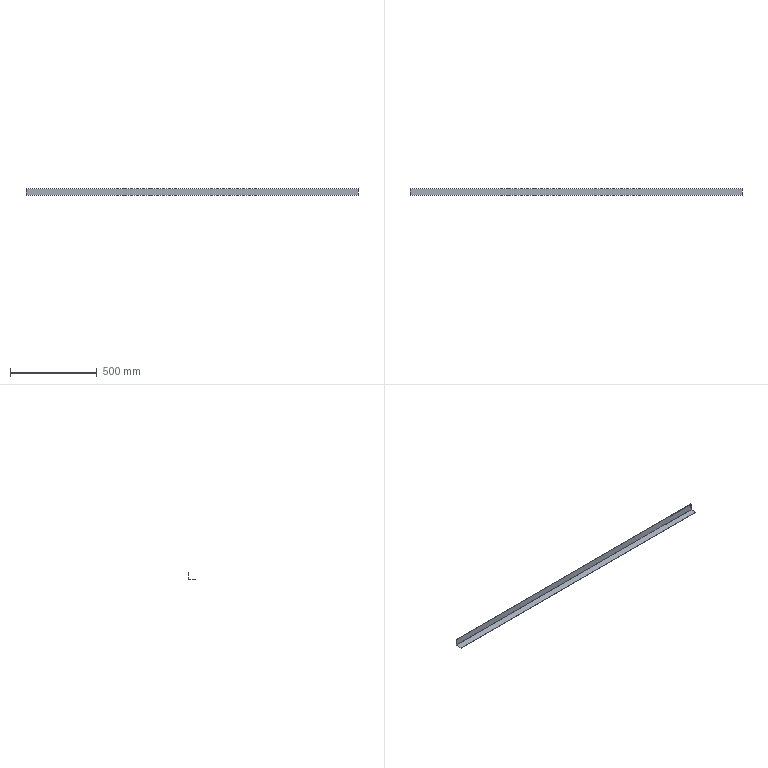Part | SolidWorks | features EdgeFlange 1, FlatPattern 1, SMBaseFlange 1, SheetMetal 1 | 1 solid | 14 faces | box 1910 x 40 x 40 mm | volume 179921 mm3 | plane 12 | cylinder 2 | commonest cylinder face diameters 0.2 x1 2.6 x1
STEP:
#1=CARTESIAN_POINT('',(-955.,18.7,0.));
#2=VERTEX_POINT('',#1);
#3=CARTESIAN_POINT('',(-955.,-20.,0.));
#4=VERTEX_POINT('',#3);
#5=CARTESIAN_POINT('',(-955.,20.,0.));
#6=DIRECTION('',(0.,-1.,0.));
#7=VECTOR('',#6,1000.);
#8=LINE('',#5,#7);
#9=EDGE_CURVE('',#2,#4,#8,.T.);
#10=ORIENTED_EDGE('',*,*,#9,.F.);
#11=CARTESIAN_POINT('',(-955.,18.7,-1.2));
#12=VERTEX_POINT('',#11);
#13=CARTESIAN_POINT('',(-955.,18.7,0.));
#14=DIRECTION('',(0.,0.,-1.));
#15=VECTOR('',#14,1000.);
#16=LINE('',#13,#15);
#17=EDGE_CURVE('',#2,#12,#16,.T.);
#18=ORIENTED_EDGE('',*,*,#17,.T.);
#19=CARTESIAN_POINT('',(-955.,-20.,-1.2));
#20=VERTEX_POINT('',#19);
#21=CARTESIAN_POINT('',(-955.,20.,-1.2));
#22=DIRECTION('',(0.,-1.,0.));
#23=VECTOR('',#22,1000.);
#24=LINE('',#21,#23);
#25=EDGE_CURVE('',#12,#20,#24,.T.);
#26=ORIENTED_EDGE('',*,*,#25,.T.);
#27=CARTESIAN_POINT('',(-955.,-20.,-1.2));
#28=DIRECTION('',(0.,0.,1.));
#29=VECTOR('',#28,1000.);
#30=LINE('',#27,#29);
#31=EDGE_CURVE('',#20,#4,#30,.T.);
#32=ORIENTED_EDGE('',*,*,#31,.T.);
#33=EDGE_LOOP('',(#10,#18,#26,#32));
#34=FACE_OUTER_BOUND('',#33,.T.);
#35=CARTESIAN_POINT('',(-955.,20.,-1.2));
#36=DIRECTION('',(-1.,0.,0.));
#37=DIRECTION('',(0.,0.,1.));
#38=AXIS2_PLACEMENT_3D('',#35,#36,#37);
#39=PLANE('',#38);
#40=ADVANCED_FACE('',(#34),#39,.T.);
#41=CARTESIAN_POINT('',(955.,18.7,-1.2));
#42=VERTEX_POINT('',#41);
#43=CARTESIAN_POINT('',(-955.,18.7,-1.2));
#44=DIRECTION('',(1.,0.,0.));
#45=VECTOR('',#44,1000.);
#46=LINE('',#43,#45);
#47=EDGE_CURVE('',#12,#42,#46,.T.);
#48=ORIENTED_EDGE('',*,*,#47,.T.);
#49=CARTESIAN_POINT('',(955.,-20.,-1.2));
#50=VERTEX_POINT('',#49);
#51=CARTESIAN_POINT('',(955.,20.,-1.2));
#52=DIRECTION('',(0.,1.,0.));
#53=VECTOR('',#52,1000.);
#54=LINE('',#51,#53);
#55=EDGE_CURVE('',#50,#42,#54,.T.);
#56=ORIENTED_EDGE('',*,*,#55,.F.);
#57=CARTESIAN_POINT('',(-955.,-20.,-1.2));
#58=DIRECTION('',(1.,0.,0.));
#59=VECTOR('',#58,1000.);
#60=LINE('',#57,#59);
#61=EDGE_CURVE('',#20,#50,#60,.T.);
#62=ORIENTED_EDGE('',*,*,#61,.F.);
#63=ORIENTED_EDGE('',*,*,#25,.F.);
#64=EDGE_LOOP('',(#48,#56,#62,#63));
#65=FACE_OUTER_BOUND('',#64,.T.);
#66=CARTESIAN_POINT('',(0.,0.,-1.2));
#67=DIRECTION('',(0.,0.,1.));
#68=DIRECTION('',(1.,0.,0.));
#69=AXIS2_PLACEMENT_3D('',#66,#67,#68);
#70=PLANE('',#69);
#71=ADVANCED_FACE('',(#65),#70,.F.);
#72=CARTESIAN_POINT('',(955.,-20.,0.));
#73=VERTEX_POINT('',#72);
#74=CARTESIAN_POINT('',(955.,18.7,0.));
#75=VERTEX_POINT('',#74);
#76=CARTESIAN_POINT('',(955.,20.,0.));
#77=DIRECTION('',(0.,1.,0.));
#78=VECTOR('',#77,1000.);
#79=LINE('',#76,#78);
#80=EDGE_CURVE('',#73,#75,#79,.T.);
#81=ORIENTED_EDGE('',*,*,#80,.T.);
#82=CARTESIAN_POINT('',(-955.,18.7,0.));
#83=DIRECTION('',(1.,0.,0.));
#84=VECTOR('',#83,1000.);
#85=LINE('',#82,#84);
#86=EDGE_CURVE('',#2,#75,#85,.T.);
#87=ORIENTED_EDGE('',*,*,#86,.F.);
#88=ORIENTED_EDGE('',*,*,#9,.T.);
#89=CARTESIAN_POINT('',(-955.,-20.,0.));
#90=DIRECTION('',(1.,0.,0.));
#91=VECTOR('',#90,1000.);
#92=LINE('',#89,#91);
#93=EDGE_CURVE('',#4,#73,#92,.T.);
#94=ORIENTED_EDGE('',*,*,#93,.T.);
#95=EDGE_LOOP('',(#81,#87,#88,#94));
#96=FACE_OUTER_BOUND('',#95,.T.);
#97=CARTESIAN_POINT('',(0.,0.,0.));
#98=DIRECTION('',(0.,0.,1.));
#99=DIRECTION('',(1.,0.,0.));
#100=AXIS2_PLACEMENT_3D('',#97,#98,#99);
#101=PLANE('',#100);
#102=ADVANCED_FACE('',(#96),#101,.T.);
#103=CARTESIAN_POINT('',(955.,18.7,0.));
#104=DIRECTION('',(0.,0.,-1.));
#105=VECTOR('',#104,1000.);
#106=LINE('',#103,#105);
#107=EDGE_CURVE('',#75,#42,#106,.T.);
#108=ORIENTED_EDGE('',*,*,#107,.F.);
#109=ORIENTED_EDGE('',*,*,#80,.F.);
#110=CARTESIAN_POINT('',(955.,-20.,-1.2));
#111=DIRECTION('',(0.,0.,1.));
#112=VECTOR('',#111,1000.);
#113=LINE('',#110,#112);
#114=EDGE_CURVE('',#50,#73,#113,.T.);
#115=ORIENTED_EDGE('',*,*,#114,.F.);
#116=ORIENTED_EDGE('',*,*,#55,.T.);
#117=EDGE_LOOP('',(#108,#109,#115,#116));
#118=FACE_OUTER_BOUND('',#117,.T.);
#119=CARTESIAN_POINT('',(955.,20.,-1.2));
#120=DIRECTION('',(1.,0.,0.));
#121=DIRECTION('',(0.,0.,-1.));
#122=AXIS2_PLACEMENT_3D('',#119,#120,#121);
#123=PLANE('',#122);
#124=ADVANCED_FACE('',(#118),#123,.T.);
#125=ORIENTED_EDGE('',*,*,#93,.F.);
#126=ORIENTED_EDGE('',*,*,#31,.F.);
#127=ORIENTED_EDGE('',*,*,#61,.T.);
#128=ORIENTED_EDGE('',*,*,#114,.T.);
#129=EDGE_LOOP('',(#125,#126,#127,#128));
#130=FACE_OUTER_BOUND('',#129,.T.);
#131=CARTESIAN_POINT('',(-955.,-20.,-1.2));
#132=DIRECTION('',(0.,-1.,0.));
#133=DIRECTION('',(0.,0.,-1.));
#134=AXIS2_PLACEMENT_3D('',#131,#132,#133);
#135=PLANE('',#134);
#136=ADVANCED_FACE('',(#130),#135,.T.);
#137=CARTESIAN_POINT('',(955.,18.8,0.1));
#138=VERTEX_POINT('',#137);
#139=CARTESIAN_POINT('',(955.,20.,0.1));
#140=VERTEX_POINT('',#139);
#141=CARTESIAN_POINT('',(955.,20.,0.1));
#142=DIRECTION('',(0.,1.,0.));
#143=VECTOR('',#142,1000.);
#144=LINE('',#141,#143);
#145=EDGE_CURVE('',#138,#140,#144,.T.);
#146=ORIENTED_EDGE('',*,*,#145,.F.);
#147=CARTESIAN_POINT('',(955.,18.7,0.1));
#148=DIRECTION('',(1.,0.,0.));
#149=DIRECTION('',(0.,0.,1.));
#150=AXIS2_PLACEMENT_3D('',#147,#148,#149);
#151=CIRCLE('',#150,0.1);
#152=EDGE_CURVE('',#75,#138,#151,.T.);
#153=ORIENTED_EDGE('',*,*,#152,.F.);
#154=ORIENTED_EDGE('',*,*,#107,.T.);
#155=CARTESIAN_POINT('',(955.,18.7,0.1));
#156=DIRECTION('',(1.,0.,0.));
#157=DIRECTION('',(0.,0.,1.));
#158=AXIS2_PLACEMENT_3D('',#155,#156,#157);
#159=CIRCLE('',#158,1.3);
#160=EDGE_CURVE('',#42,#140,#159,.T.);
#161=ORIENTED_EDGE('',*,*,#160,.T.);
#162=EDGE_LOOP('',(#146,#153,#154,#161));
#163=FACE_OUTER_BOUND('',#162,.T.);
#164=CARTESIAN_POINT('',(955.,18.7,0.1));
#165=DIRECTION('',(1.,0.,0.));
#166=DIRECTION('',(0.,0.,-1.));
#167=AXIS2_PLACEMENT_3D('',#164,#165,#166);
#168=PLANE('',#167);
#169=ADVANCED_FACE('',(#163),#168,.T.);
#170=CARTESIAN_POINT('',(-955.,18.8,0.1));
#171=VERTEX_POINT('',#170);
#172=CARTESIAN_POINT('',(-955.,18.7,0.1));
#173=DIRECTION('',(-1.,0.,0.));
#174=DIRECTION('',(0.,0.,1.));
#175=AXIS2_PLACEMENT_3D('',#172,#173,#174);
#176=CIRCLE('',#175,0.1);
#177=EDGE_CURVE('',#171,#2,#176,.T.);
#178=ORIENTED_EDGE('',*,*,#177,.F.);
#179=CARTESIAN_POINT('',(-955.,20.,0.1));
#180=VERTEX_POINT('',#179);
#181=CARTESIAN_POINT('',(-955.,18.8,0.1));
#182=DIRECTION('',(0.,1.,0.));
#183=VECTOR('',#182,1000.);
#184=LINE('',#181,#183);
#185=EDGE_CURVE('',#171,#180,#184,.T.);
#186=ORIENTED_EDGE('',*,*,#185,.T.);
#187=CARTESIAN_POINT('',(-955.,18.7,0.1));
#188=DIRECTION('',(-1.,0.,0.));
#189=DIRECTION('',(0.,0.,1.));
#190=AXIS2_PLACEMENT_3D('',#187,#188,#189);
#191=CIRCLE('',#190,1.3);
#192=EDGE_CURVE('',#180,#12,#191,.T.);
#193=ORIENTED_EDGE('',*,*,#192,.T.);
#194=ORIENTED_EDGE('',*,*,#17,.F.);
#195=EDGE_LOOP('',(#178,#186,#193,#194));
#196=FACE_OUTER_BOUND('',#195,.T.);
#197=CARTESIAN_POINT('',(-955.,18.7,0.1));
#198=DIRECTION('',(1.,0.,0.));
#199=DIRECTION('',(0.,0.,-1.));
#200=AXIS2_PLACEMENT_3D('',#197,#198,#199);
#201=PLANE('',#200);
#202=ADVANCED_FACE('',(#196),#201,.F.);
#203=ORIENTED_EDGE('',*,*,#47,.F.);
#204=ORIENTED_EDGE('',*,*,#192,.F.);
#205=CARTESIAN_POINT('',(955.,20.,0.1));
#206=DIRECTION('',(1.,0.,0.));
#207=VECTOR('',#206,1000.);
#208=LINE('',#205,#207);
#209=EDGE_CURVE('',#180,#140,#208,.T.);
#210=ORIENTED_EDGE('',*,*,#209,.T.);
#211=ORIENTED_EDGE('',*,*,#160,.F.);
#212=EDGE_LOOP('',(#203,#204,#210,#211));
#213=FACE_OUTER_BOUND('',#212,.T.);
#214=CARTESIAN_POINT('',(-955.,18.7,0.1));
#215=DIRECTION('',(-1.,0.,0.));
#216=DIRECTION('',(0.,1.,0.));
#217=AXIS2_PLACEMENT_3D('',#214,#215,#216);
#218=CYLINDRICAL_SURFACE('',#217,1.3);
#219=ADVANCED_FACE('',(#213),#218,.T.);
#220=ORIENTED_EDGE('',*,*,#86,.T.);
#221=ORIENTED_EDGE('',*,*,#152,.T.);
#222=CARTESIAN_POINT('',(955.,18.8,0.1));
#223=DIRECTION('',(-1.,0.,0.));
#224=VECTOR('',#223,1000.);
#225=LINE('',#222,#224);
#226=EDGE_CURVE('',#138,#171,#225,.T.);
#227=ORIENTED_EDGE('',*,*,#226,.T.);
#228=ORIENTED_EDGE('',*,*,#177,.T.);
#229=EDGE_LOOP('',(#220,#221,#227,#228));
#230=FACE_OUTER_BOUND('',#229,.T.);
#231=CARTESIAN_POINT('',(-955.,18.7,0.1));
#232=DIRECTION('',(-1.,0.,0.));
#233=DIRECTION('',(0.,1.,0.));
#234=AXIS2_PLACEMENT_3D('',#231,#232,#233);
#235=CYLINDRICAL_SURFACE('',#234,0.1);
#236=ADVANCED_FACE('',(#230),#235,.F.);
#237=ORIENTED_EDGE('',*,*,#185,.F.);
#238=CARTESIAN_POINT('',(-955.,18.8,38.8));
#239=VERTEX_POINT('',#238);
#240=CARTESIAN_POINT('',(-955.,18.8,38.8));
#241=DIRECTION('',(0.,0.,1.));
#242=VECTOR('',#241,1000.);
#243=LINE('',#240,#242);
#244=EDGE_CURVE('',#171,#239,#243,.T.);
#245=ORIENTED_EDGE('',*,*,#244,.T.);
#246=CARTESIAN_POINT('',(-955.,20.,38.8));
#247=VERTEX_POINT('',#246);
#248=CARTESIAN_POINT('',(-955.,20.,38.8));
#249=DIRECTION('',(0.,-1.,0.));
#250=VECTOR('',#249,1000.);
#251=LINE('',#248,#250);
#252=EDGE_CURVE('',#247,#239,#251,.T.);
#253=ORIENTED_EDGE('',*,*,#252,.F.);
#254=CARTESIAN_POINT('',(-955.,20.,0.));
#255=DIRECTION('',(0.,0.,1.));
#256=VECTOR('',#255,1000.);
#257=LINE('',#254,#256);
#258=EDGE_CURVE('',#180,#247,#257,.T.);
#259=ORIENTED_EDGE('',*,*,#258,.F.);
#260=EDGE_LOOP('',(#237,#245,#253,#259));
#261=FACE_OUTER_BOUND('',#260,.T.);
#262=CARTESIAN_POINT('',(-955.,20.,38.8));
#263=DIRECTION('',(1.,0.,0.));
#264=DIRECTION('',(0.,0.,-1.));
#265=AXIS2_PLACEMENT_3D('',#262,#263,#264);
#266=PLANE('',#265);
#267=ADVANCED_FACE('',(#261),#266,.F.);
#268=ORIENTED_EDGE('',*,*,#145,.T.);
#269=CARTESIAN_POINT('',(955.,20.,38.8));
#270=VERTEX_POINT('',#269);
#271=CARTESIAN_POINT('',(955.,20.,0.));
#272=DIRECTION('',(0.,0.,-1.));
#273=VECTOR('',#272,1000.);
#274=LINE('',#271,#273);
#275=EDGE_CURVE('',#270,#140,#274,.T.);
#276=ORIENTED_EDGE('',*,*,#275,.F.);
#277=CARTESIAN_POINT('',(955.,18.8,38.8));
#278=VERTEX_POINT('',#277);
#279=CARTESIAN_POINT('',(955.,20.,38.8));
#280=DIRECTION('',(0.,-1.,0.));
#281=VECTOR('',#280,1000.);
#282=LINE('',#279,#281);
#283=EDGE_CURVE('',#270,#278,#282,.T.);
#284=ORIENTED_EDGE('',*,*,#283,.T.);
#285=CARTESIAN_POINT('',(955.,18.8,0.));
#286=DIRECTION('',(0.,0.,-1.));
#287=VECTOR('',#286,1000.);
#288=LINE('',#285,#287);
#289=EDGE_CURVE('',#278,#138,#288,.T.);
#290=ORIENTED_EDGE('',*,*,#289,.T.);
#291=EDGE_LOOP('',(#268,#276,#284,#290));
#292=FACE_OUTER_BOUND('',#291,.T.);
#293=CARTESIAN_POINT('',(955.,20.,0.));
#294=DIRECTION('',(-1.,0.,0.));
#295=DIRECTION('',(0.,0.,1.));
#296=AXIS2_PLACEMENT_3D('',#293,#294,#295);
#297=PLANE('',#296);
#298=ADVANCED_FACE('',(#292),#297,.F.);
#299=ORIENTED_EDGE('',*,*,#209,.F.);
#300=ORIENTED_EDGE('',*,*,#258,.T.);
#301=CARTESIAN_POINT('',(0.,20.,38.8));
#302=DIRECTION('',(1.,0.,0.));
#303=VECTOR('',#302,1000.);
#304=LINE('',#301,#303);
#305=EDGE_CURVE('',#247,#270,#304,.T.);
#306=ORIENTED_EDGE('',*,*,#305,.T.);
#307=ORIENTED_EDGE('',*,*,#275,.T.);
#308=EDGE_LOOP('',(#299,#300,#306,#307));
#309=FACE_OUTER_BOUND('',#308,.T.);
#310=CARTESIAN_POINT('',(0.,20.,0.));
#311=DIRECTION('',(0.,-1.,0.));
#312=DIRECTION('',(0.,0.,-1.));
#313=AXIS2_PLACEMENT_3D('',#310,#311,#312);
#314=PLANE('',#313);
#315=ADVANCED_FACE('',(#309),#314,.F.);
#316=ORIENTED_EDGE('',*,*,#244,.F.);
#317=ORIENTED_EDGE('',*,*,#226,.F.);
#318=ORIENTED_EDGE('',*,*,#289,.F.);
#319=CARTESIAN_POINT('',(955.,18.8,38.8));
#320=DIRECTION('',(1.,0.,0.));
#321=VECTOR('',#320,1000.);
#322=LINE('',#319,#321);
#323=EDGE_CURVE('',#239,#278,#322,.T.);
#324=ORIENTED_EDGE('',*,*,#323,.F.);
#325=EDGE_LOOP('',(#316,#317,#318,#324));
#326=FACE_OUTER_BOUND('',#325,.T.);
#327=CARTESIAN_POINT('',(0.,18.8,0.));
#328=DIRECTION('',(0.,-1.,0.));
#329=DIRECTION('',(0.,0.,-1.));
#330=AXIS2_PLACEMENT_3D('',#327,#328,#329);
#331=PLANE('',#330);
#332=ADVANCED_FACE('',(#326),#331,.T.);
#333=ORIENTED_EDGE('',*,*,#323,.T.);
#334=ORIENTED_EDGE('',*,*,#283,.F.);
#335=ORIENTED_EDGE('',*,*,#305,.F.);
#336=ORIENTED_EDGE('',*,*,#252,.T.);
#337=EDGE_LOOP('',(#333,#334,#335,#336));
#338=FACE_OUTER_BOUND('',#337,.T.);
#339=CARTESIAN_POINT('',(955.,20.,38.8));
#340=DIRECTION('',(0.,0.,-1.));
#341=DIRECTION('',(0.,1.,0.));
#342=AXIS2_PLACEMENT_3D('',#339,#340,#341);
#343=PLANE('',#342);
#344=ADVANCED_FACE('',(#338),#343,.F.);
#345=CLOSED_SHELL('',(#40,#71,#102,#124,#136,#169,#202,#219,#236,#267,#298,#315,#332,#344));
#346=MANIFOLD_SOLID_BREP('',#345);
#347=CARTESIAN_POINT('',(0.,0.,0.));
#348=DIRECTION('',(0.,0.,1.));
#349=DIRECTION('',(1.,0.,0.));
#350=AXIS2_PLACEMENT_3D('',#347,#348,#349);
#351=(LENGTH_UNIT()NAMED_UNIT(*)SI_UNIT(.MILLI.,.METRE.));
#352=UNCERTAINTY_MEASURE_WITH_UNIT(LENGTH_MEASURE(0.00001),#351,'','');
#353=(NAMED_UNIT(*)PLANE_ANGLE_UNIT()SI_UNIT($,.RADIAN.));
#354=(NAMED_UNIT(*)SI_UNIT($,.STERADIAN.)SOLID_ANGLE_UNIT());
#355=(GEOMETRIC_REPRESENTATION_CONTEXT(3)GLOBAL_UNCERTAINTY_ASSIGNED_CONTEXT((#352))GLOBAL_UNIT_ASSIGNED_CONTEXT((#351,#353,#354))REPRESENTATION_CONTEXT('',''));
#356=ADVANCED_BREP_SHAPE_REPRESENTATION('',(#346,#350),#355);